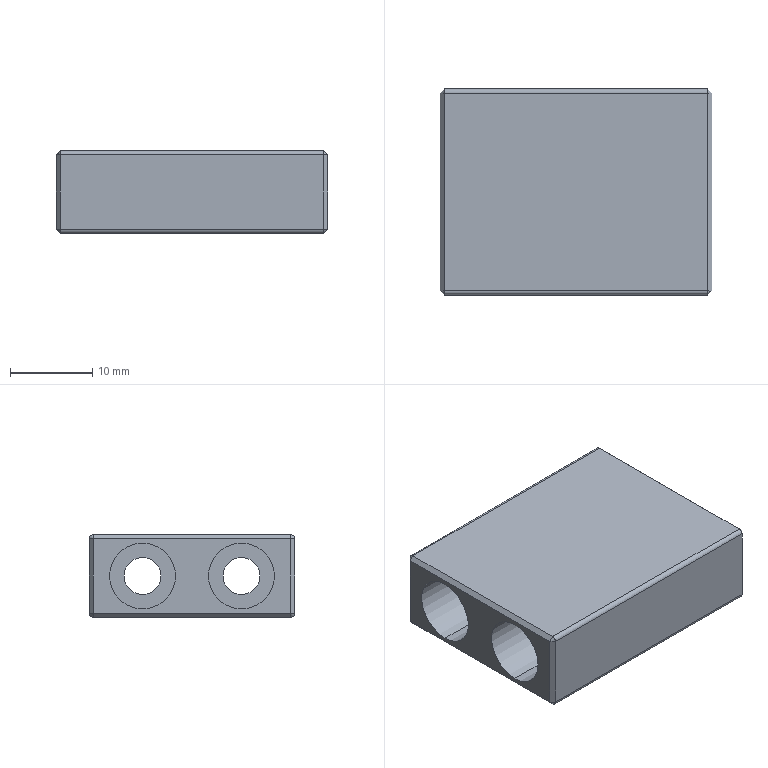Part | SolidWorks | features BaseBody 1 | 1 solid | 36 faces | box 33 x 25 x 10 mm | volume 5939 mm3 | plane 16 | cylinder 12 | cone 8 | commonest cylinder face diameters 1 x4 4.5 x4 8 x4
STEP:
#1=CARTESIAN_POINT('',(-846.13,707.797,333.482));
#2=VERTEX_POINT('',#1);
#3=CARTESIAN_POINT('',(-846.13,707.797,341.482));
#4=VERTEX_POINT('',#3);
#5=CARTESIAN_POINT('',(-846.13,707.797,337.482));
#6=DIRECTION('',(-1.,-0.000001544,0.));
#7=DIRECTION('',(0.,0.,-1.));
#8=AXIS2_PLACEMENT_3D('',#5,#6,#7);
#9=CIRCLE('',#8,4.);
#10=EDGE_CURVE('',#2,#4,#9,.T.);
#11=ORIENTED_EDGE('',*,*,#10,.T.);
#12=CARTESIAN_POINT('',(-828.13,707.797,341.482));
#13=VERTEX_POINT('',#12);
#14=CARTESIAN_POINT('',(-828.13,707.797,341.482));
#15=DIRECTION('',(-1.,-0.000001544,0.));
#16=VECTOR('',#15,1000.);
#17=LINE('',#14,#16);
#18=EDGE_CURVE('',#13,#4,#17,.T.);
#19=ORIENTED_EDGE('',*,*,#18,.F.);
#20=CARTESIAN_POINT('',(-828.13,707.797,333.482));
#21=VERTEX_POINT('',#20);
#22=CARTESIAN_POINT('',(-828.13,707.797,337.482));
#23=DIRECTION('',(1.,0.000001544,0.));
#24=DIRECTION('',(0.,0.,1.));
#25=AXIS2_PLACEMENT_3D('',#22,#23,#24);
#26=CIRCLE('',#25,4.);
#27=EDGE_CURVE('',#13,#21,#26,.T.);
#28=ORIENTED_EDGE('',*,*,#27,.T.);
#29=CARTESIAN_POINT('',(-846.13,707.797,333.482));
#30=DIRECTION('',(1.,0.000001544,0.));
#31=VECTOR('',#30,1000.);
#32=LINE('',#29,#31);
#33=EDGE_CURVE('',#2,#21,#32,.T.);
#34=ORIENTED_EDGE('',*,*,#33,.F.);
#35=EDGE_LOOP('',(#11,#19,#28,#34));
#36=FACE_OUTER_BOUND('',#35,.T.);
#37=CARTESIAN_POINT('',(-846.13,707.797,337.482));
#38=DIRECTION('',(-1.,-0.000001544,0.));
#39=DIRECTION('',(0.,0.,-1.));
#40=AXIS2_PLACEMENT_3D('',#37,#38,#39);
#41=CYLINDRICAL_SURFACE('',#40,4.);
#42=ADVANCED_FACE('',(#36),#41,.F.);
#43=ORIENTED_EDGE('',*,*,#18,.T.);
#44=CARTESIAN_POINT('',(-846.13,707.797,337.482));
#45=DIRECTION('',(-1.,-0.000001544,0.));
#46=DIRECTION('',(0.,0.,1.));
#47=AXIS2_PLACEMENT_3D('',#44,#45,#46);
#48=CIRCLE('',#47,4.);
#49=EDGE_CURVE('',#4,#2,#48,.T.);
#50=ORIENTED_EDGE('',*,*,#49,.T.);
#51=ORIENTED_EDGE('',*,*,#33,.T.);
#52=CARTESIAN_POINT('',(-828.13,707.797,337.482));
#53=DIRECTION('',(1.,0.000001544,0.));
#54=DIRECTION('',(0.,0.,-1.));
#55=AXIS2_PLACEMENT_3D('',#52,#53,#54);
#56=CIRCLE('',#55,4.);
#57=EDGE_CURVE('',#21,#13,#56,.T.);
#58=ORIENTED_EDGE('',*,*,#57,.T.);
#59=EDGE_LOOP('',(#43,#50,#51,#58));
#60=FACE_OUTER_BOUND('',#59,.T.);
#61=CARTESIAN_POINT('',(-846.13,707.797,337.482));
#62=DIRECTION('',(-1.,-0.000001544,0.));
#63=DIRECTION('',(0.,0.,-1.));
#64=AXIS2_PLACEMENT_3D('',#61,#62,#63);
#65=CYLINDRICAL_SURFACE('',#64,4.);
#66=ADVANCED_FACE('',(#60),#65,.F.);
#67=ORIENTED_EDGE('',*,*,#57,.F.);
#68=ORIENTED_EDGE('',*,*,#27,.F.);
#69=EDGE_LOOP('',(#67,#68));
#70=FACE_OUTER_BOUND('',#69,.T.);
#71=CARTESIAN_POINT('',(-828.13,707.797,339.732));
#72=VERTEX_POINT('',#71);
#73=CARTESIAN_POINT('',(-828.13,707.797,335.232));
#74=VERTEX_POINT('',#73);
#75=CARTESIAN_POINT('',(-828.13,707.797,337.482));
#76=DIRECTION('',(-1.,-0.000001544,0.));
#77=DIRECTION('',(0.,0.,1.));
#78=AXIS2_PLACEMENT_3D('',#75,#76,#77);
#79=CIRCLE('',#78,2.25);
#80=EDGE_CURVE('',#72,#74,#79,.T.);
#81=ORIENTED_EDGE('',*,*,#80,.F.);
#82=CARTESIAN_POINT('',(-828.13,707.797,337.482));
#83=DIRECTION('',(-1.,-0.000001544,0.));
#84=DIRECTION('',(0.,0.,-1.));
#85=AXIS2_PLACEMENT_3D('',#82,#83,#84);
#86=CIRCLE('',#85,2.25);
#87=EDGE_CURVE('',#74,#72,#86,.T.);
#88=ORIENTED_EDGE('',*,*,#87,.F.);
#89=EDGE_LOOP('',(#81,#88));
#90=FACE_BOUND('',#89,.T.);
#91=CARTESIAN_POINT('',(-828.13,710.047,337.482));
#92=DIRECTION('',(1.,0.000001544,0.));
#93=DIRECTION('',(0.,0.,1.));
#94=AXIS2_PLACEMENT_3D('',#91,#92,#93);
#95=PLANE('',#94);
#96=ADVANCED_FACE('',(#70,#90),#95,.F.);
#97=ORIENTED_EDGE('',*,*,#87,.T.);
#98=CARTESIAN_POINT('',(-813.13,707.797,339.732));
#99=VERTEX_POINT('',#98);
#100=CARTESIAN_POINT('',(-828.13,707.797,339.732));
#101=DIRECTION('',(1.,0.000001544,0.));
#102=VECTOR('',#101,1000.);
#103=LINE('',#100,#102);
#104=EDGE_CURVE('',#72,#99,#103,.T.);
#105=ORIENTED_EDGE('',*,*,#104,.T.);
#106=CARTESIAN_POINT('',(-813.13,707.797,335.232));
#107=VERTEX_POINT('',#106);
#108=CARTESIAN_POINT('',(-813.13,707.797,337.482));
#109=DIRECTION('',(1.,0.000001544,0.));
#110=DIRECTION('',(0.,0.,1.));
#111=AXIS2_PLACEMENT_3D('',#108,#109,#110);
#112=CIRCLE('',#111,2.25);
#113=EDGE_CURVE('',#99,#107,#112,.T.);
#114=ORIENTED_EDGE('',*,*,#113,.T.);
#115=CARTESIAN_POINT('',(-813.13,707.797,335.232));
#116=DIRECTION('',(-1.,-0.000001544,0.));
#117=VECTOR('',#116,1000.);
#118=LINE('',#115,#117);
#119=EDGE_CURVE('',#107,#74,#118,.T.);
#120=ORIENTED_EDGE('',*,*,#119,.T.);
#121=EDGE_LOOP('',(#97,#105,#114,#120));
#122=FACE_OUTER_BOUND('',#121,.T.);
#123=CARTESIAN_POINT('',(-846.13,707.797,337.482));
#124=DIRECTION('',(-1.,-0.000001544,0.));
#125=DIRECTION('',(0.,0.,-1.));
#126=AXIS2_PLACEMENT_3D('',#123,#124,#125);
#127=CYLINDRICAL_SURFACE('',#126,2.25);
#128=ADVANCED_FACE('',(#122),#127,.F.);
#129=ORIENTED_EDGE('',*,*,#104,.F.);
#130=ORIENTED_EDGE('',*,*,#80,.T.);
#131=ORIENTED_EDGE('',*,*,#119,.F.);
#132=CARTESIAN_POINT('',(-813.13,707.797,337.482));
#133=DIRECTION('',(1.,0.000001544,0.));
#134=DIRECTION('',(0.,0.,-1.));
#135=AXIS2_PLACEMENT_3D('',#132,#133,#134);
#136=CIRCLE('',#135,2.25);
#137=EDGE_CURVE('',#107,#99,#136,.T.);
#138=ORIENTED_EDGE('',*,*,#137,.T.);
#139=EDGE_LOOP('',(#129,#130,#131,#138));
#140=FACE_OUTER_BOUND('',#139,.T.);
#141=CARTESIAN_POINT('',(-846.13,707.797,337.482));
#142=DIRECTION('',(-1.,-0.000001544,0.));
#143=DIRECTION('',(0.,0.,-1.));
#144=AXIS2_PLACEMENT_3D('',#141,#142,#143);
#145=CYLINDRICAL_SURFACE('',#144,2.25);
#146=ADVANCED_FACE('',(#140),#145,.F.);
#147=CARTESIAN_POINT('',(-813.13,689.797,332.982));
#148=VERTEX_POINT('',#147);
#149=CARTESIAN_POINT('',(-813.13,713.797,332.982));
#150=VERTEX_POINT('',#149);
#151=CARTESIAN_POINT('',(-813.13,689.797,332.982));
#152=DIRECTION('',(-0.000001544,1.,0.));
#153=VECTOR('',#152,1000.);
#154=LINE('',#151,#153);
#155=EDGE_CURVE('',#148,#150,#154,.T.);
#156=ORIENTED_EDGE('',*,*,#155,.T.);
#157=CARTESIAN_POINT('',(-813.13,713.797,341.982));
#158=VERTEX_POINT('',#157);
#159=CARTESIAN_POINT('',(-813.13,713.797,332.982));
#160=DIRECTION('',(0.,0.,1.));
#161=VECTOR('',#160,1000.);
#162=LINE('',#159,#161);
#163=EDGE_CURVE('',#150,#158,#162,.T.);
#164=ORIENTED_EDGE('',*,*,#163,.T.);
#165=CARTESIAN_POINT('',(-813.13,689.797,341.982));
#166=VERTEX_POINT('',#165);
#167=CARTESIAN_POINT('',(-813.13,689.797,341.982));
#168=DIRECTION('',(-0.000001544,1.,0.));
#169=VECTOR('',#168,1000.);
#170=LINE('',#167,#169);
#171=EDGE_CURVE('',#166,#158,#170,.T.);
#172=ORIENTED_EDGE('',*,*,#171,.F.);
#173=CARTESIAN_POINT('',(-813.13,689.797,332.982));
#174=DIRECTION('',(0.,0.,1.));
#175=VECTOR('',#174,1000.);
#176=LINE('',#173,#175);
#177=EDGE_CURVE('',#148,#166,#176,.T.);
#178=ORIENTED_EDGE('',*,*,#177,.F.);
#179=EDGE_LOOP('',(#156,#164,#172,#178));
#180=FACE_OUTER_BOUND('',#179,.T.);
#181=CARTESIAN_POINT('',(-813.13,695.797,335.232));
#182=VERTEX_POINT('',#181);
#183=CARTESIAN_POINT('',(-813.13,695.797,339.732));
#184=VERTEX_POINT('',#183);
#185=CARTESIAN_POINT('',(-813.13,695.797,337.482));
#186=DIRECTION('',(1.,0.000001544,0.));
#187=DIRECTION('',(0.,0.,-1.));
#188=AXIS2_PLACEMENT_3D('',#185,#186,#187);
#189=CIRCLE('',#188,2.25);
#190=EDGE_CURVE('',#182,#184,#189,.T.);
#191=ORIENTED_EDGE('',*,*,#190,.F.);
#192=CARTESIAN_POINT('',(-813.13,695.797,337.482));
#193=DIRECTION('',(1.,0.000001544,0.));
#194=DIRECTION('',(0.,0.,1.));
#195=AXIS2_PLACEMENT_3D('',#192,#193,#194);
#196=CIRCLE('',#195,2.25);
#197=EDGE_CURVE('',#184,#182,#196,.T.);
#198=ORIENTED_EDGE('',*,*,#197,.F.);
#199=EDGE_LOOP('',(#191,#198));
#200=FACE_BOUND('',#199,.T.);
#201=ORIENTED_EDGE('',*,*,#137,.F.);
#202=ORIENTED_EDGE('',*,*,#113,.F.);
#203=EDGE_LOOP('',(#201,#202));
#204=FACE_BOUND('',#203,.T.);
#205=CARTESIAN_POINT('',(-813.13,714.297,332.482));
#206=DIRECTION('',(-1.,-0.000001544,0.));
#207=DIRECTION('',(0.000001544,-1.,0.));
#208=AXIS2_PLACEMENT_3D('',#205,#206,#207);
#209=PLANE('',#208);
#210=ADVANCED_FACE('',(#180,#200,#204),#209,.F.);
#211=CARTESIAN_POINT('',(-813.63,689.297,341.982));
#212=VERTEX_POINT('',#211);
#213=CARTESIAN_POINT('',(-813.13,689.797,341.982));
#214=DIRECTION('',(-0.7071,-0.7071,0.));
#215=VECTOR('',#214,1000.);
#216=LINE('',#213,#215);
#217=EDGE_CURVE('',#166,#212,#216,.T.);
#218=ORIENTED_EDGE('',*,*,#217,.T.);
#219=CARTESIAN_POINT('',(-813.63,689.297,332.982));
#220=VERTEX_POINT('',#219);
#221=CARTESIAN_POINT('',(-813.63,689.297,341.982));
#222=DIRECTION('',(0.,0.,-1.));
#223=VECTOR('',#222,1000.);
#224=LINE('',#221,#223);
#225=EDGE_CURVE('',#212,#220,#224,.T.);
#226=ORIENTED_EDGE('',*,*,#225,.T.);
#227=CARTESIAN_POINT('',(-813.63,689.297,332.982));
#228=DIRECTION('',(0.7071,0.7071,0.));
#229=VECTOR('',#228,1000.);
#230=LINE('',#227,#229);
#231=EDGE_CURVE('',#220,#148,#230,.T.);
#232=ORIENTED_EDGE('',*,*,#231,.T.);
#233=ORIENTED_EDGE('',*,*,#177,.T.);
#234=EDGE_LOOP('',(#218,#226,#232,#233));
#235=FACE_OUTER_BOUND('',#234,.T.);
#236=CARTESIAN_POINT('',(-813.63,689.297,332.482));
#237=DIRECTION('',(-0.7071,0.7071,0.));
#238=DIRECTION('',(0.,0.,-1.));
#239=AXIS2_PLACEMENT_3D('',#236,#237,#238);
#240=PLANE('',#239);
#241=ADVANCED_FACE('',(#235),#240,.F.);
#242=ORIENTED_EDGE('',*,*,#231,.F.);
#243=CARTESIAN_POINT('',(-813.63,689.797,332.482));
#244=VERTEX_POINT('',#243);
#245=CARTESIAN_POINT('',(-813.63,689.797,332.982));
#246=DIRECTION('',(-1.,-0.000001544,0.));
#247=DIRECTION('',(0.,0.,-1.));
#248=AXIS2_PLACEMENT_3D('',#245,#246,#247);
#249=CIRCLE('',#248,0.5);
#250=EDGE_CURVE('',#244,#220,#249,.T.);
#251=ORIENTED_EDGE('',*,*,#250,.F.);
#252=CARTESIAN_POINT('',(-813.13,689.797,332.982));
#253=DIRECTION('',(-0.7071,-0.000001092,-0.7071));
#254=VECTOR('',#253,1000.);
#255=LINE('',#252,#254);
#256=EDGE_CURVE('',#148,#244,#255,.T.);
#257=ORIENTED_EDGE('',*,*,#256,.F.);
#258=EDGE_LOOP('',(#242,#251,#257));
#259=FACE_OUTER_BOUND('',#258,.T.);
#260=CARTESIAN_POINT('',(-813.398,689.797,332.982));
#261=DIRECTION('',(-1.,-0.000001544,0.));
#262=DIRECTION('',(-0.000001544,1.,0.));
#263=AXIS2_PLACEMENT_3D('',#260,#261,#262);
#264=CONICAL_SURFACE('',#263,0.2681,0.7854);
#265=ADVANCED_FACE('',(#259),#264,.T.);
#266=ORIENTED_EDGE('',*,*,#256,.T.);
#267=CARTESIAN_POINT('',(-813.63,713.797,332.482));
#268=VERTEX_POINT('',#267);
#269=CARTESIAN_POINT('',(-813.63,689.797,332.482));
#270=DIRECTION('',(-0.000001544,1.,0.));
#271=VECTOR('',#270,1000.);
#272=LINE('',#269,#271);
#273=EDGE_CURVE('',#244,#268,#272,.T.);
#274=ORIENTED_EDGE('',*,*,#273,.T.);
#275=CARTESIAN_POINT('',(-813.63,713.797,332.482));
#276=DIRECTION('',(0.7071,0.000001092,0.7071));
#277=VECTOR('',#276,1000.);
#278=LINE('',#275,#277);
#279=EDGE_CURVE('',#268,#150,#278,.T.);
#280=ORIENTED_EDGE('',*,*,#279,.T.);
#281=ORIENTED_EDGE('',*,*,#155,.F.);
#282=EDGE_LOOP('',(#266,#274,#280,#281));
#283=FACE_OUTER_BOUND('',#282,.T.);
#284=CARTESIAN_POINT('',(-813.63,701.797,332.482));
#285=DIRECTION('',(0.7071,0.000001092,-0.7071));
#286=DIRECTION('',(0.000001544,-1.,0.));
#287=AXIS2_PLACEMENT_3D('',#284,#285,#286);
#288=PLANE('',#287);
#289=ADVANCED_FACE('',(#283),#288,.T.);
#290=ORIENTED_EDGE('',*,*,#279,.F.);
#291=CARTESIAN_POINT('',(-813.63,714.297,332.982));
#292=VERTEX_POINT('',#291);
#293=CARTESIAN_POINT('',(-813.63,713.797,332.982));
#294=DIRECTION('',(-1.,-0.000001544,0.));
#295=DIRECTION('',(-0.000001544,1.,0.));
#296=AXIS2_PLACEMENT_3D('',#293,#294,#295);
#297=CIRCLE('',#296,0.5);
#298=EDGE_CURVE('',#292,#268,#297,.T.);
#299=ORIENTED_EDGE('',*,*,#298,.F.);
#300=CARTESIAN_POINT('',(-813.13,713.797,332.982));
#301=DIRECTION('',(-0.7071,0.7071,0.));
#302=VECTOR('',#301,1000.);
#303=LINE('',#300,#302);
#304=EDGE_CURVE('',#150,#292,#303,.T.);
#305=ORIENTED_EDGE('',*,*,#304,.F.);
#306=EDGE_LOOP('',(#290,#299,#305));
#307=FACE_OUTER_BOUND('',#306,.T.);
#308=CARTESIAN_POINT('',(-813.398,713.797,332.982));
#309=DIRECTION('',(-1.,-0.000001544,0.));
#310=DIRECTION('',(-0.000001544,1.,0.));
#311=AXIS2_PLACEMENT_3D('',#308,#309,#310);
#312=CONICAL_SURFACE('',#311,0.2681,0.7854);
#313=ADVANCED_FACE('',(#307),#312,.T.);
#314=CARTESIAN_POINT('',(-813.63,714.297,341.982));
#315=VERTEX_POINT('',#314);
#316=CARTESIAN_POINT('',(-813.63,714.297,341.982));
#317=DIRECTION('',(0.7071,-0.7071,0.));
#318=VECTOR('',#317,1000.);
#319=LINE('',#316,#318);
#320=EDGE_CURVE('',#315,#158,#319,.T.);
#321=ORIENTED_EDGE('',*,*,#320,.T.);
#322=ORIENTED_EDGE('',*,*,#163,.F.);
#323=ORIENTED_EDGE('',*,*,#304,.T.);
#324=CARTESIAN_POINT('',(-813.63,714.297,332.982));
#325=DIRECTION('',(0.,0.,1.));
#326=VECTOR('',#325,1000.);
#327=LINE('',#324,#326);
#328=EDGE_CURVE('',#292,#315,#327,.T.);
#329=ORIENTED_EDGE('',*,*,#328,.T.);
#330=EDGE_LOOP('',(#321,#322,#323,#329));
#331=FACE_OUTER_BOUND('',#330,.T.);
#332=CARTESIAN_POINT('',(-813.13,713.797,332.482));
#333=DIRECTION('',(-0.7071,-0.7071,0.));
#334=DIRECTION('',(0.,0.,-1.));
#335=AXIS2_PLACEMENT_3D('',#332,#333,#334);
#336=PLANE('',#335);
#337=ADVANCED_FACE('',(#331),#336,.F.);
#338=CARTESIAN_POINT('',(-845.63,714.297,332.982));
#339=VERTEX_POINT('',#338);
#340=CARTESIAN_POINT('',(-813.63,714.297,332.982));
#341=DIRECTION('',(-1.,-0.000001544,0.));
#342=VECTOR('',#341,1000.);
#343=LINE('',#340,#342);
#344=EDGE_CURVE('',#292,#339,#343,.T.);
#345=ORIENTED_EDGE('',*,*,#344,.T.);
#346=CARTESIAN_POINT('',(-845.63,714.297,341.982));
#347=VERTEX_POINT('',#346);
#348=CARTESIAN_POINT('',(-845.63,714.297,341.982));
#349=DIRECTION('',(0.,0.,-1.));
#350=VECTOR('',#349,1000.);
#351=LINE('',#348,#350);
#352=EDGE_CURVE('',#347,#339,#351,.T.);
#353=ORIENTED_EDGE('',*,*,#352,.F.);
#354=CARTESIAN_POINT('',(-845.63,714.297,341.982));
#355=DIRECTION('',(1.,0.000001544,0.));
#356=VECTOR('',#355,1000.);
#357=LINE('',#354,#356);
#358=EDGE_CURVE('',#347,#315,#357,.T.);
#359=ORIENTED_EDGE('',*,*,#358,.T.);
#360=ORIENTED_EDGE('',*,*,#328,.F.);
#361=EDGE_LOOP('',(#345,#353,#359,#360));
#362=FACE_OUTER_BOUND('',#361,.T.);
#363=CARTESIAN_POINT('',(-813.13,714.297,332.482));
#364=DIRECTION('',(0.000001544,-1.,0.));
#365=DIRECTION('',(0.,0.,-1.));
#366=AXIS2_PLACEMENT_3D('',#363,#364,#365);
#367=PLANE('',#366);
#368=ADVANCED_FACE('',(#362),#367,.F.);
#369=ORIENTED_EDGE('',*,*,#358,.F.);
#370=CARTESIAN_POINT('',(-845.63,713.797,342.482));
#371=VERTEX_POINT('',#370);
#372=CARTESIAN_POINT('',(-845.63,713.797,341.982));
#373=DIRECTION('',(1.,0.000001544,0.));
#374=DIRECTION('',(-0.000001544,1.,0.));
#375=AXIS2_PLACEMENT_3D('',#372,#373,#374);
#376=CIRCLE('',#375,0.5);
#377=EDGE_CURVE('',#347,#371,#376,.T.);
#378=ORIENTED_EDGE('',*,*,#377,.T.);
#379=CARTESIAN_POINT('',(-813.63,713.797,342.482));
#380=VERTEX_POINT('',#379);
#381=CARTESIAN_POINT('',(-813.63,713.797,342.482));
#382=DIRECTION('',(-1.,-0.000001544,0.));
#383=VECTOR('',#382,1000.);
#384=LINE('',#381,#383);
#385=EDGE_CURVE('',#380,#371,#384,.T.);
#386=ORIENTED_EDGE('',*,*,#385,.F.);
#387=CARTESIAN_POINT('',(-813.63,713.797,341.982));
#388=DIRECTION('',(-1.,-0.000001544,0.));
#389=DIRECTION('',(0.,0.,1.));
#390=AXIS2_PLACEMENT_3D('',#387,#388,#389);
#391=CIRCLE('',#390,0.5);
#392=EDGE_CURVE('',#380,#315,#391,.T.);
#393=ORIENTED_EDGE('',*,*,#392,.T.);
#394=EDGE_LOOP('',(#369,#378,#386,#393));
#395=FACE_OUTER_BOUND('',#394,.T.);
#396=CARTESIAN_POINT('',(-813.13,713.797,341.982));
#397=DIRECTION('',(1.,0.000001544,0.));
#398=DIRECTION('',(0.,0.,1.));
#399=AXIS2_PLACEMENT_3D('',#396,#397,#398);
#400=CYLINDRICAL_SURFACE('',#399,0.5);
#401=ADVANCED_FACE('',(#395),#400,.T.);
#402=CARTESIAN_POINT('',(-813.13,713.797,341.982));
#403=DIRECTION('',(-0.7071,-0.000001092,0.7071));
#404=VECTOR('',#403,1000.);
#405=LINE('',#402,#404);
#406=EDGE_CURVE('',#158,#380,#405,.T.);
#407=ORIENTED_EDGE('',*,*,#406,.F.);
#408=ORIENTED_EDGE('',*,*,#320,.F.);
#409=ORIENTED_EDGE('',*,*,#392,.F.);
#410=EDGE_LOOP('',(#407,#408,#409));
#411=FACE_OUTER_BOUND('',#410,.T.);
#412=CARTESIAN_POINT('',(-813.398,713.797,341.982));
#413=DIRECTION('',(-1.,-0.000001544,0.));
#414=DIRECTION('',(-0.000001544,1.,0.));
#415=AXIS2_PLACEMENT_3D('',#412,#413,#414);
#416=CONICAL_SURFACE('',#415,0.2681,0.7854);
#417=ADVANCED_FACE('',(#411),#416,.T.);
#418=CARTESIAN_POINT('',(-813.63,689.797,342.482));
#419=VERTEX_POINT('',#418);
#420=CARTESIAN_POINT('',(-813.63,689.797,342.482));
#421=DIRECTION('',(0.7071,0.000001092,-0.7071));
#422=VECTOR('',#421,1000.);
#423=LINE('',#420,#422);
#424=EDGE_CURVE('',#419,#166,#423,.T.);
#425=ORIENTED_EDGE('',*,*,#424,.T.);
#426=ORIENTED_EDGE('',*,*,#171,.T.);
#427=ORIENTED_EDGE('',*,*,#406,.T.);
#428=CARTESIAN_POINT('',(-813.63,713.797,342.482));
#429=DIRECTION('',(0.000001544,-1.,0.));
#430=VECTOR('',#429,1000.);
#431=LINE('',#428,#430);
#432=EDGE_CURVE('',#380,#419,#431,.T.);
#433=ORIENTED_EDGE('',*,*,#432,.T.);
#434=EDGE_LOOP('',(#425,#426,#427,#433));
#435=FACE_OUTER_BOUND('',#434,.T.);
#436=CARTESIAN_POINT('',(-813.13,714.297,341.982));
#437=DIRECTION('',(-0.7071,-0.000001092,-0.7071));
#438=DIRECTION('',(-0.000001544,1.,0.));
#439=AXIS2_PLACEMENT_3D('',#436,#437,#438);
#440=PLANE('',#439);
#441=ADVANCED_FACE('',(#435),#440,.F.);
#442=ORIENTED_EDGE('',*,*,#385,.T.);
#443=CARTESIAN_POINT('',(-845.63,689.797,342.482));
#444=VERTEX_POINT('',#443);
#445=CARTESIAN_POINT('',(-845.63,689.797,342.482));
#446=DIRECTION('',(-0.000001544,1.,0.));
#447=VECTOR('',#446,1000.);
#448=LINE('',#445,#447);
#449=EDGE_CURVE('',#444,#371,#448,.T.);
#450=ORIENTED_EDGE('',*,*,#449,.F.);
#451=CARTESIAN_POINT('',(-845.63,689.797,342.482));
#452=DIRECTION('',(1.,0.000001544,0.));
#453=VECTOR('',#452,1000.);
#454=LINE('',#451,#453);
#455=EDGE_CURVE('',#444,#419,#454,.T.);
#456=ORIENTED_EDGE('',*,*,#455,.T.);
#457=ORIENTED_EDGE('',*,*,#432,.F.);
#458=EDGE_LOOP('',(#442,#450,#456,#457));
#459=FACE_OUTER_BOUND('',#458,.T.);
#460=CARTESIAN_POINT('',(-829.63,701.797,342.482));
#461=DIRECTION('',(0.,0.,-1.));
#462=DIRECTION('',(1.,0.000001544,0.));
#463=AXIS2_PLACEMENT_3D('',#460,#461,#462);
#464=PLANE('',#463);
#465=ADVANCED_FACE('',(#459),#464,.F.);
#466=ORIENTED_EDGE('',*,*,#455,.F.);
#467=CARTESIAN_POINT('',(-845.63,689.297,341.982));
#468=VERTEX_POINT('',#467);
#469=CARTESIAN_POINT('',(-845.63,689.797,341.982));
#470=DIRECTION('',(1.,0.000001544,0.));
#471=DIRECTION('',(0.,0.,1.));
#472=AXIS2_PLACEMENT_3D('',#469,#470,#471);
#473=CIRCLE('',#472,0.5);
#474=EDGE_CURVE('',#444,#468,#473,.T.);
#475=ORIENTED_EDGE('',*,*,#474,.T.);
#476=CARTESIAN_POINT('',(-813.63,689.297,341.982));
#477=DIRECTION('',(-1.,-0.000001544,0.));
#478=VECTOR('',#477,1000.);
#479=LINE('',#476,#478);
#480=EDGE_CURVE('',#212,#468,#479,.T.);
#481=ORIENTED_EDGE('',*,*,#480,.F.);
#482=CARTESIAN_POINT('',(-813.63,689.797,341.982));
#483=DIRECTION('',(-1.,-0.000001544,0.));
#484=DIRECTION('',(0.000001544,-1.,0.));
#485=AXIS2_PLACEMENT_3D('',#482,#483,#484);
#486=CIRCLE('',#485,0.5);
#487=EDGE_CURVE('',#212,#419,#486,.T.);
#488=ORIENTED_EDGE('',*,*,#487,.T.);
#489=EDGE_LOOP('',(#466,#475,#481,#488));
#490=FACE_OUTER_BOUND('',#489,.T.);
#491=CARTESIAN_POINT('',(-813.13,689.797,341.982));
#492=DIRECTION('',(-1.,-0.000001544,0.));
#493=DIRECTION('',(0.,0.,-1.));
#494=AXIS2_PLACEMENT_3D('',#491,#492,#493);
#495=CYLINDRICAL_SURFACE('',#494,0.5);
#496=ADVANCED_FACE('',(#490),#495,.T.);
#497=ORIENTED_EDGE('',*,*,#217,.F.);
#498=ORIENTED_EDGE('',*,*,#424,.F.);
#499=ORIENTED_EDGE('',*,*,#487,.F.);
#500=EDGE_LOOP('',(#497,#498,#499));
#501=FACE_OUTER_BOUND('',#500,.T.);
#502=CARTESIAN_POINT('',(-813.398,689.797,341.982));
#503=DIRECTION('',(-1.,-0.000001544,0.));
#504=DIRECTION('',(0.,0.,-1.));
#505=AXIS2_PLACEMENT_3D('',#502,#503,#504);
#506=CONICAL_SURFACE('',#505,0.2681,0.7854);
#507=ADVANCED_FACE('',(#501),#506,.T.);
#508=ORIENTED_EDGE('',*,*,#480,.T.);
#509=CARTESIAN_POINT('',(-845.63,689.297,332.982));
#510=VERTEX_POINT('',#509);
#511=CARTESIAN_POINT('',(-845.63,689.297,341.982));
#512=DIRECTION('',(0.,0.,-1.));
#513=VECTOR('',#512,1000.);
#514=LINE('',#511,#513);
#515=EDGE_CURVE('',#468,#510,#514,.T.);
#516=ORIENTED_EDGE('',*,*,#515,.T.);
#517=CARTESIAN_POINT('',(-845.63,689.297,332.982));
#518=DIRECTION('',(1.,0.000001544,0.));
#519=VECTOR('',#518,1000.);
#520=LINE('',#517,#519);
#521=EDGE_CURVE('',#510,#220,#520,.T.);
#522=ORIENTED_EDGE('',*,*,#521,.T.);
#523=ORIENTED_EDGE('',*,*,#225,.F.);
#524=EDGE_LOOP('',(#508,#516,#522,#523));
#525=FACE_OUTER_BOUND('',#524,.T.);
#526=CARTESIAN_POINT('',(-813.13,689.297,332.482));
#527=DIRECTION('',(-0.000001544,1.,0.));
#528=DIRECTION('',(0.,0.,1.));
#529=AXIS2_PLACEMENT_3D('',#526,#527,#528);
#530=PLANE('',#529);
#531=ADVANCED_FACE('',(#525),#530,.F.);
#532=ORIENTED_EDGE('',*,*,#521,.F.);
#533=CARTESIAN_POINT('',(-845.63,689.797,332.482));
#534=VERTEX_POINT('',#533);
#535=CARTESIAN_POINT('',(-845.63,689.797,332.982));
#536=DIRECTION('',(1.,0.000001544,0.));
#537=DIRECTION('',(0.000001544,-1.,0.));
#538=AXIS2_PLACEMENT_3D('',#535,#536,#537);
#539=CIRCLE('',#538,0.5);
#540=EDGE_CURVE('',#510,#534,#539,.T.);
#541=ORIENTED_EDGE('',*,*,#540,.T.);
#542=CARTESIAN_POINT('',(-813.63,689.797,332.482));
#543=DIRECTION('',(-1.,-0.000001544,0.));
#544=VECTOR('',#543,1000.);
#545=LINE('',#542,#544);
#546=EDGE_CURVE('',#244,#534,#545,.T.);
#547=ORIENTED_EDGE('',*,*,#546,.F.);
#548=ORIENTED_EDGE('',*,*,#250,.T.);
#549=EDGE_LOOP('',(#532,#541,#547,#548));
#550=FACE_OUTER_BOUND('',#549,.T.);
#551=CARTESIAN_POINT('',(-829.63,689.797,332.982));
#552=DIRECTION('',(1.,0.000001544,0.));
#553=DIRECTION('',(0.,0.,1.));
#554=AXIS2_PLACEMENT_3D('',#551,#552,#553);
#555=CYLINDRICAL_SURFACE('',#554,0.5);
#556=ADVANCED_FACE('',(#550),#555,.T.);
#557=ORIENTED_EDGE('',*,*,#546,.T.);
#558=CARTESIAN_POINT('',(-845.63,713.797,332.482));
#559=VERTEX_POINT('',#558);
#560=CARTESIAN_POINT('',(-845.63,689.797,332.482));
#561=DIRECTION('',(-0.000001544,1.,0.));
#562=VECTOR('',#561,1000.);
#563=LINE('',#560,#562);
#564=EDGE_CURVE('',#534,#559,#563,.T.);
#565=ORIENTED_EDGE('',*,*,#564,.T.);
#566=CARTESIAN_POINT('',(-845.63,713.797,332.482));
#567=DIRECTION('',(1.,0.000001544,0.));
#568=VECTOR('',#567,1000.);
#569=LINE('',#566,#568);
#570=EDGE_CURVE('',#559,#268,#569,.T.);
#571=ORIENTED_EDGE('',*,*,#570,.T.);
#572=ORIENTED_EDGE('',*,*,#273,.F.);
#573=EDGE_LOOP('',(#557,#565,#571,#572));
#574=FACE_OUTER_BOUND('',#573,.T.);
#575=CARTESIAN_POINT('',(-829.63,701.797,332.482));
#576=DIRECTION('',(0.,0.,-1.));
#577=DIRECTION('',(1.,0.000001544,0.));
#578=AXIS2_PLACEMENT_3D('',#575,#576,#577);
#579=PLANE('',#578);
#580=ADVANCED_FACE('',(#574),#579,.T.);
#581=ORIENTED_EDGE('',*,*,#570,.F.);
#582=CARTESIAN_POINT('',(-845.63,713.797,332.982));
#583=DIRECTION('',(1.,0.000001544,0.));
#584=DIRECTION('',(0.,0.,-1.));
#585=AXIS2_PLACEMENT_3D('',#582,#583,#584);
#586=CIRCLE('',#585,0.5);
#587=EDGE_CURVE('',#559,#339,#586,.T.);
#588=ORIENTED_EDGE('',*,*,#587,.T.);
#589=ORIENTED_EDGE('',*,*,#344,.F.);
#590=ORIENTED_EDGE('',*,*,#298,.T.);
#591=EDGE_LOOP('',(#581,#588,#589,#590));
#592=FACE_OUTER_BOUND('',#591,.T.);
#593=CARTESIAN_POINT('',(-829.63,713.797,332.982));
#594=DIRECTION('',(-1.,-0.000001544,0.));
#595=DIRECTION('',(0.,0.,-1.));
#596=AXIS2_PLACEMENT_3D('',#593,#594,#595);
#597=CYLINDRICAL_SURFACE('',#596,0.5);
#598=ADVANCED_FACE('',(#592),#597,.T.);
#599=CARTESIAN_POINT('',(-846.13,713.797,332.982));
#600=VERTEX_POINT('',#599);
#601=CARTESIAN_POINT('',(-845.63,714.297,332.982));
#602=DIRECTION('',(-0.7071,-0.7071,0.));
#603=VECTOR('',#602,1000.);
#604=LINE('',#601,#603);
#605=EDGE_CURVE('',#339,#600,#604,.T.);
#606=ORIENTED_EDGE('',*,*,#605,.F.);
#607=ORIENTED_EDGE('',*,*,#587,.F.);
#608=CARTESIAN_POINT('',(-846.13,713.797,332.982));
#609=DIRECTION('',(0.7071,0.000001092,-0.7071));
#610=VECTOR('',#609,1000.);
#611=LINE('',#608,#610);
#612=EDGE_CURVE('',#600,#559,#611,.T.);
#613=ORIENTED_EDGE('',*,*,#612,.F.);
#614=EDGE_LOOP('',(#606,#607,#613));
#615=FACE_OUTER_BOUND('',#614,.T.);
#616=CARTESIAN_POINT('',(-845.862,713.797,332.982));
#617=DIRECTION('',(1.,0.000001544,0.));
#618=DIRECTION('',(0.,0.,-1.));
#619=AXIS2_PLACEMENT_3D('',#616,#617,#618);
#620=CONICAL_SURFACE('',#619,0.2681,0.7854);
#621=ADVANCED_FACE('',(#615),#620,.T.);
#622=CARTESIAN_POINT('',(-846.13,689.797,332.982));
#623=VERTEX_POINT('',#622);
#624=CARTESIAN_POINT('',(-845.63,689.797,332.482));
#625=DIRECTION('',(-0.7071,-0.000001092,0.7071));
#626=VECTOR('',#625,1000.);
#627=LINE('',#624,#626);
#628=EDGE_CURVE('',#534,#623,#627,.T.);
#629=ORIENTED_EDGE('',*,*,#628,.T.);
#630=CARTESIAN_POINT('',(-846.13,689.797,332.982));
#631=DIRECTION('',(-0.000001544,1.,0.));
#632=VECTOR('',#631,1000.);
#633=LINE('',#630,#632);
#634=EDGE_CURVE('',#623,#600,#633,.T.);
#635=ORIENTED_EDGE('',*,*,#634,.T.);
#636=ORIENTED_EDGE('',*,*,#612,.T.);
#637=ORIENTED_EDGE('',*,*,#564,.F.);
#638=EDGE_LOOP('',(#629,#635,#636,#637));
#639=FACE_OUTER_BOUND('',#638,.T.);
#640=CARTESIAN_POINT('',(-845.63,701.797,332.482));
#641=DIRECTION('',(-0.7071,-0.000001092,-0.7071));
#642=DIRECTION('',(-0.000001544,1.,0.));
#643=AXIS2_PLACEMENT_3D('',#640,#641,#642);
#644=PLANE('',#643);
#645=ADVANCED_FACE('',(#639),#644,.T.);
#646=CARTESIAN_POINT('',(-846.13,713.797,341.982));
#647=VERTEX_POINT('',#646);
#648=CARTESIAN_POINT('',(-846.13,713.797,332.982));
#649=DIRECTION('',(0.,0.,1.));
#650=VECTOR('',#649,1000.);
#651=LINE('',#648,#650);
#652=EDGE_CURVE('',#600,#647,#651,.T.);
#653=ORIENTED_EDGE('',*,*,#652,.F.);
#654=ORIENTED_EDGE('',*,*,#634,.F.);
#655=CARTESIAN_POINT('',(-846.13,689.797,341.982));
#656=VERTEX_POINT('',#655);
#657=CARTESIAN_POINT('',(-846.13,689.797,341.982));
#658=DIRECTION('',(0.,0.,-1.));
#659=VECTOR('',#658,1000.);
#660=LINE('',#657,#659);
#661=EDGE_CURVE('',#656,#623,#660,.T.);
#662=ORIENTED_EDGE('',*,*,#661,.F.);
#663=CARTESIAN_POINT('',(-846.13,713.797,341.982));
#664=DIRECTION('',(0.000001544,-1.,0.));
#665=VECTOR('',#664,1000.);
#666=LINE('',#663,#665);
#667=EDGE_CURVE('',#647,#656,#666,.T.);
#668=ORIENTED_EDGE('',*,*,#667,.F.);
#669=EDGE_LOOP('',(#653,#654,#662,#668));
#670=FACE_OUTER_BOUND('',#669,.T.);
#671=CARTESIAN_POINT('',(-846.13,695.797,341.482));
#672=VERTEX_POINT('',#671);
#673=CARTESIAN_POINT('',(-846.13,695.797,333.482));
#674=VERTEX_POINT('',#673);
#675=CARTESIAN_POINT('',(-846.13,695.797,337.482));
#676=DIRECTION('',(-1.,-0.000001544,0.));
#677=DIRECTION('',(0.,0.,1.));
#678=AXIS2_PLACEMENT_3D('',#675,#676,#677);
#679=CIRCLE('',#678,4.);
#680=EDGE_CURVE('',#672,#674,#679,.T.);
#681=ORIENTED_EDGE('',*,*,#680,.F.);
#682=CARTESIAN_POINT('',(-846.13,695.797,337.482));
#683=DIRECTION('',(-1.,-0.000001544,0.));
#684=DIRECTION('',(0.,0.,-1.));
#685=AXIS2_PLACEMENT_3D('',#682,#683,#684);
#686=CIRCLE('',#685,4.);
#687=EDGE_CURVE('',#674,#672,#686,.T.);
#688=ORIENTED_EDGE('',*,*,#687,.F.);
#689=EDGE_LOOP('',(#681,#688));
#690=FACE_BOUND('',#689,.T.);
#691=ORIENTED_EDGE('',*,*,#49,.F.);
#692=ORIENTED_EDGE('',*,*,#10,.F.);
#693=EDGE_LOOP('',(#691,#692));
#694=FACE_BOUND('',#693,.T.);
#695=CARTESIAN_POINT('',(-846.13,714.297,332.482));
#696=DIRECTION('',(1.,0.000001544,0.));
#697=DIRECTION('',(0.,0.,1.));
#698=AXIS2_PLACEMENT_3D('',#695,#696,#697);
#699=PLANE('',#698);
#700=ADVANCED_FACE('',(#670,#690,#694),#699,.F.);
#701=CARTESIAN_POINT('',(-845.63,713.797,342.482));
#702=DIRECTION('',(-0.7071,-0.000001092,-0.7071));
#703=VECTOR('',#702,1000.);
#704=LINE('',#701,#703);
#705=EDGE_CURVE('',#371,#647,#704,.T.);
#706=ORIENTED_EDGE('',*,*,#705,.T.);
#707=ORIENTED_EDGE('',*,*,#667,.T.);
#708=CARTESIAN_POINT('',(-846.13,689.797,341.982));
#709=DIRECTION('',(0.7071,0.000001092,0.7071));
#710=VECTOR('',#709,1000.);
#711=LINE('',#708,#710);
#712=EDGE_CURVE('',#656,#444,#711,.T.);
#713=ORIENTED_EDGE('',*,*,#712,.T.);
#714=ORIENTED_EDGE('',*,*,#449,.T.);
#715=EDGE_LOOP('',(#706,#707,#713,#714));
#716=FACE_OUTER_BOUND('',#715,.T.);
#717=CARTESIAN_POINT('',(-846.13,714.297,341.982));
#718=DIRECTION('',(0.7071,0.000001092,-0.7071));
#719=DIRECTION('',(0.000001544,-1.,0.));
#720=AXIS2_PLACEMENT_3D('',#717,#718,#719);
#721=PLANE('',#720);
#722=ADVANCED_FACE('',(#716),#721,.F.);
#723=ORIENTED_EDGE('',*,*,#712,.F.);
#724=CARTESIAN_POINT('',(-845.63,689.297,341.982));
#725=DIRECTION('',(-0.7071,0.7071,0.));
#726=VECTOR('',#725,1000.);
#727=LINE('',#724,#726);
#728=EDGE_CURVE('',#468,#656,#727,.T.);
#729=ORIENTED_EDGE('',*,*,#728,.F.);
#730=ORIENTED_EDGE('',*,*,#474,.F.);
#731=EDGE_LOOP('',(#723,#729,#730));
#732=FACE_OUTER_BOUND('',#731,.T.);
#733=CARTESIAN_POINT('',(-845.862,689.797,341.982));
#734=DIRECTION('',(1.,0.000001544,0.));
#735=DIRECTION('',(0.,0.,1.));
#736=AXIS2_PLACEMENT_3D('',#733,#734,#735);
#737=CONICAL_SURFACE('',#736,0.2681,0.7854);
#738=ADVANCED_FACE('',(#732),#737,.T.);
#739=ORIENTED_EDGE('',*,*,#728,.T.);
#740=ORIENTED_EDGE('',*,*,#661,.T.);
#741=CARTESIAN_POINT('',(-846.13,689.797,332.982));
#742=DIRECTION('',(0.7071,-0.7071,0.));
#743=VECTOR('',#742,1000.);
#744=LINE('',#741,#743);
#745=EDGE_CURVE('',#623,#510,#744,.T.);
#746=ORIENTED_EDGE('',*,*,#745,.T.);
#747=ORIENTED_EDGE('',*,*,#515,.F.);
#748=EDGE_LOOP('',(#739,#740,#746,#747));
#749=FACE_OUTER_BOUND('',#748,.T.);
#750=CARTESIAN_POINT('',(-846.13,689.797,332.482));
#751=DIRECTION('',(0.7071,0.7071,0.));
#752=DIRECTION('',(0.,0.,-1.));
#753=AXIS2_PLACEMENT_3D('',#750,#751,#752);
#754=PLANE('',#753);
#755=ADVANCED_FACE('',(#749),#754,.F.);
#756=ORIENTED_EDGE('',*,*,#745,.F.);
#757=ORIENTED_EDGE('',*,*,#628,.F.);
#758=ORIENTED_EDGE('',*,*,#540,.F.);
#759=EDGE_LOOP('',(#756,#757,#758));
#760=FACE_OUTER_BOUND('',#759,.T.);
#761=CARTESIAN_POINT('',(-845.862,689.797,332.982));
#762=DIRECTION('',(1.,0.000001544,0.));
#763=DIRECTION('',(0.,0.,-1.));
#764=AXIS2_PLACEMENT_3D('',#761,#762,#763);
#765=CONICAL_SURFACE('',#764,0.2681,0.7854);
#766=ADVANCED_FACE('',(#760),#765,.T.);
#767=ORIENTED_EDGE('',*,*,#705,.F.);
#768=ORIENTED_EDGE('',*,*,#377,.F.);
#769=CARTESIAN_POINT('',(-846.13,713.797,341.982));
#770=DIRECTION('',(0.7071,0.7071,0.));
#771=VECTOR('',#770,1000.);
#772=LINE('',#769,#771);
#773=EDGE_CURVE('',#647,#347,#772,.T.);
#774=ORIENTED_EDGE('',*,*,#773,.F.);
#775=EDGE_LOOP('',(#767,#768,#774));
#776=FACE_OUTER_BOUND('',#775,.T.);
#777=CARTESIAN_POINT('',(-845.862,713.797,341.982));
#778=DIRECTION('',(1.,0.000001544,0.));
#779=DIRECTION('',(0.,0.,-1.));
#780=AXIS2_PLACEMENT_3D('',#777,#778,#779);
#781=CONICAL_SURFACE('',#780,0.2681,0.7854);
#782=ADVANCED_FACE('',(#776),#781,.T.);
#783=ORIENTED_EDGE('',*,*,#773,.T.);
#784=ORIENTED_EDGE('',*,*,#352,.T.);
#785=ORIENTED_EDGE('',*,*,#605,.T.);
#786=ORIENTED_EDGE('',*,*,#652,.T.);
#787=EDGE_LOOP('',(#783,#784,#785,#786));
#788=FACE_OUTER_BOUND('',#787,.T.);
#789=CARTESIAN_POINT('',(-845.63,714.297,332.482));
#790=DIRECTION('',(0.7071,-0.7071,0.));
#791=DIRECTION('',(0.,0.,-1.));
#792=AXIS2_PLACEMENT_3D('',#789,#790,#791);
#793=PLANE('',#792);
#794=ADVANCED_FACE('',(#788),#793,.F.);
#795=ORIENTED_EDGE('',*,*,#687,.T.);
#796=CARTESIAN_POINT('',(-828.13,695.797,341.482));
#797=VERTEX_POINT('',#796);
#798=CARTESIAN_POINT('',(-846.13,695.797,341.482));
#799=DIRECTION('',(1.,0.000001544,0.));
#800=VECTOR('',#799,1000.);
#801=LINE('',#798,#800);
#802=EDGE_CURVE('',#672,#797,#801,.T.);
#803=ORIENTED_EDGE('',*,*,#802,.T.);
#804=CARTESIAN_POINT('',(-828.13,695.797,333.482));
#805=VERTEX_POINT('',#804);
#806=CARTESIAN_POINT('',(-828.13,695.797,337.482));
#807=DIRECTION('',(1.,0.000001544,0.));
#808=DIRECTION('',(0.,0.,1.));
#809=AXIS2_PLACEMENT_3D('',#806,#807,#808);
#810=CIRCLE('',#809,4.);
#811=EDGE_CURVE('',#797,#805,#810,.T.);
#812=ORIENTED_EDGE('',*,*,#811,.T.);
#813=CARTESIAN_POINT('',(-828.13,695.797,333.482));
#814=DIRECTION('',(-1.,-0.000001544,0.));
#815=VECTOR('',#814,1000.);
#816=LINE('',#813,#815);
#817=EDGE_CURVE('',#805,#674,#816,.T.);
#818=ORIENTED_EDGE('',*,*,#817,.T.);
#819=EDGE_LOOP('',(#795,#803,#812,#818));
#820=FACE_OUTER_BOUND('',#819,.T.);
#821=CARTESIAN_POINT('',(-846.13,695.797,337.482));
#822=DIRECTION('',(-1.,-0.000001544,0.));
#823=DIRECTION('',(0.,0.,-1.));
#824=AXIS2_PLACEMENT_3D('',#821,#822,#823);
#825=CYLINDRICAL_SURFACE('',#824,4.);
#826=ADVANCED_FACE('',(#820),#825,.F.);
#827=ORIENTED_EDGE('',*,*,#802,.F.);
#828=ORIENTED_EDGE('',*,*,#680,.T.);
#829=ORIENTED_EDGE('',*,*,#817,.F.);
#830=CARTESIAN_POINT('',(-828.13,695.797,337.482));
#831=DIRECTION('',(1.,0.000001544,0.));
#832=DIRECTION('',(0.,0.,-1.));
#833=AXIS2_PLACEMENT_3D('',#830,#831,#832);
#834=CIRCLE('',#833,4.);
#835=EDGE_CURVE('',#805,#797,#834,.T.);
#836=ORIENTED_EDGE('',*,*,#835,.T.);
#837=EDGE_LOOP('',(#827,#828,#829,#836));
#838=FACE_OUTER_BOUND('',#837,.T.);
#839=CARTESIAN_POINT('',(-846.13,695.797,337.482));
#840=DIRECTION('',(-1.,-0.000001544,0.));
#841=DIRECTION('',(0.,0.,-1.));
#842=AXIS2_PLACEMENT_3D('',#839,#840,#841);
#843=CYLINDRICAL_SURFACE('',#842,4.);
#844=ADVANCED_FACE('',(#838),#843,.F.);
#845=ORIENTED_EDGE('',*,*,#835,.F.);
#846=ORIENTED_EDGE('',*,*,#811,.F.);
#847=EDGE_LOOP('',(#845,#846));
#848=FACE_OUTER_BOUND('',#847,.T.);
#849=CARTESIAN_POINT('',(-828.13,695.797,339.732));
#850=VERTEX_POINT('',#849);
#851=CARTESIAN_POINT('',(-828.13,695.797,335.232));
#852=VERTEX_POINT('',#851);
#853=CARTESIAN_POINT('',(-828.13,695.797,337.482));
#854=DIRECTION('',(-1.,-0.000001544,0.));
#855=DIRECTION('',(0.,0.,1.));
#856=AXIS2_PLACEMENT_3D('',#853,#854,#855);
#857=CIRCLE('',#856,2.25);
#858=EDGE_CURVE('',#850,#852,#857,.T.);
#859=ORIENTED_EDGE('',*,*,#858,.F.);
#860=CARTESIAN_POINT('',(-828.13,695.797,337.482));
#861=DIRECTION('',(-1.,-0.000001544,0.));
#862=DIRECTION('',(0.,0.,-1.));
#863=AXIS2_PLACEMENT_3D('',#860,#861,#862);
#864=CIRCLE('',#863,2.25);
#865=EDGE_CURVE('',#852,#850,#864,.T.);
#866=ORIENTED_EDGE('',*,*,#865,.F.);
#867=EDGE_LOOP('',(#859,#866));
#868=FACE_BOUND('',#867,.T.);
#869=CARTESIAN_POINT('',(-828.13,698.047,337.482));
#870=DIRECTION('',(1.,0.000001544,0.));
#871=DIRECTION('',(0.,0.,1.));
#872=AXIS2_PLACEMENT_3D('',#869,#870,#871);
#873=PLANE('',#872);
#874=ADVANCED_FACE('',(#848,#868),#873,.F.);
#875=ORIENTED_EDGE('',*,*,#865,.T.);
#876=CARTESIAN_POINT('',(-828.13,695.797,339.732));
#877=DIRECTION('',(1.,0.000001544,0.));
#878=VECTOR('',#877,1000.);
#879=LINE('',#876,#878);
#880=EDGE_CURVE('',#850,#184,#879,.T.);
#881=ORIENTED_EDGE('',*,*,#880,.T.);
#882=ORIENTED_EDGE('',*,*,#197,.T.);
#883=CARTESIAN_POINT('',(-813.13,695.797,335.232));
#884=DIRECTION('',(-1.,-0.000001544,0.));
#885=VECTOR('',#884,1000.);
#886=LINE('',#883,#885);
#887=EDGE_CURVE('',#182,#852,#886,.T.);
#888=ORIENTED_EDGE('',*,*,#887,.T.);
#889=EDGE_LOOP('',(#875,#881,#882,#888));
#890=FACE_OUTER_BOUND('',#889,.T.);
#891=CARTESIAN_POINT('',(-846.13,695.797,337.482));
#892=DIRECTION('',(-1.,-0.000001544,0.));
#893=DIRECTION('',(0.,0.,-1.));
#894=AXIS2_PLACEMENT_3D('',#891,#892,#893);
#895=CYLINDRICAL_SURFACE('',#894,2.25);
#896=ADVANCED_FACE('',(#890),#895,.F.);
#897=ORIENTED_EDGE('',*,*,#880,.F.);
#898=ORIENTED_EDGE('',*,*,#858,.T.);
#899=ORIENTED_EDGE('',*,*,#887,.F.);
#900=ORIENTED_EDGE('',*,*,#190,.T.);
#901=EDGE_LOOP('',(#897,#898,#899,#900));
#902=FACE_OUTER_BOUND('',#901,.T.);
#903=CARTESIAN_POINT('',(-846.13,695.797,337.482));
#904=DIRECTION('',(-1.,-0.000001544,0.));
#905=DIRECTION('',(0.,0.,-1.));
#906=AXIS2_PLACEMENT_3D('',#903,#904,#905);
#907=CYLINDRICAL_SURFACE('',#906,2.25);
#908=ADVANCED_FACE('',(#902),#907,.F.);
#909=CLOSED_SHELL('',(#42,#66,#96,#128,#146,#210,#241,#265,#289,#313,#337,#368,#401,#417,#441,#465,#496,#507,#531,#556,#580,#598,#621,#645,#700,#722,#738,#755,#766,#782,#794,#826,#844,#874,#896,#908));
#910=MANIFOLD_SOLID_BREP('',#909);
#911=CARTESIAN_POINT('',(0.,0.,0.));
#912=DIRECTION('',(0.,0.,1.));
#913=DIRECTION('',(1.,0.,0.));
#914=AXIS2_PLACEMENT_3D('',#911,#912,#913);
#915=(LENGTH_UNIT()NAMED_UNIT(*)SI_UNIT(.MILLI.,.METRE.));
#916=UNCERTAINTY_MEASURE_WITH_UNIT(LENGTH_MEASURE(0.00001),#915,'','');
#917=(NAMED_UNIT(*)PLANE_ANGLE_UNIT()SI_UNIT($,.RADIAN.));
#918=(NAMED_UNIT(*)SI_UNIT($,.STERADIAN.)SOLID_ANGLE_UNIT());
#919=(GEOMETRIC_REPRESENTATION_CONTEXT(3)GLOBAL_UNCERTAINTY_ASSIGNED_CONTEXT((#916))GLOBAL_UNIT_ASSIGNED_CONTEXT((#915,#917,#918))REPRESENTATION_CONTEXT('',''));
#920=ADVANCED_BREP_SHAPE_REPRESENTATION('',(#910,#914),#919);